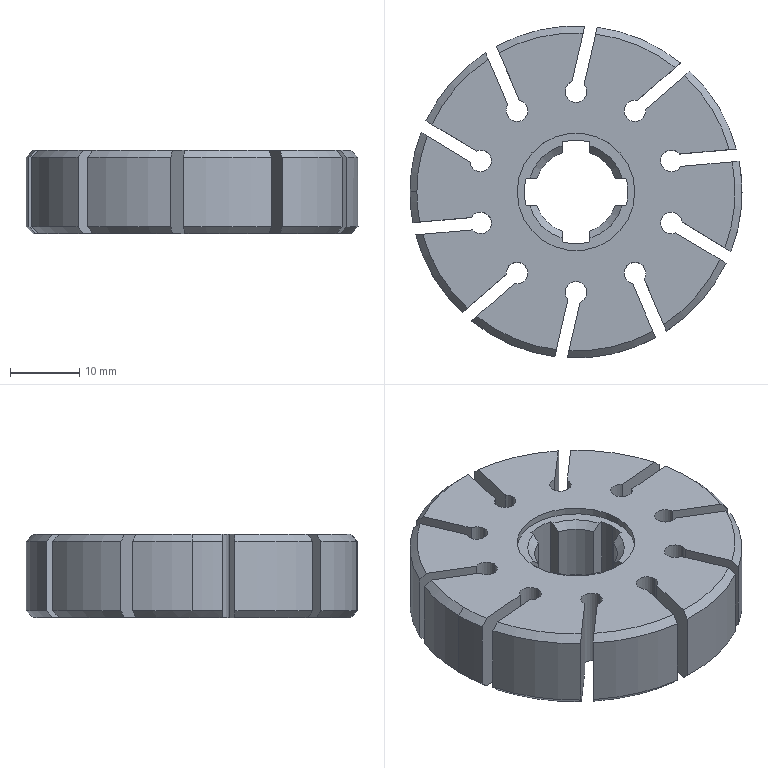Part | SolidWorks | features ICE 5, Chamfer 2, CirPattern 1, Extrusion 1 | 1 solid | 110 faces | box 48 x 48 x 12 mm | volume 17049 mm3 | cylinder 48 | plane 32 | cone 30 | commonest cylinder face diameters 3.12 x24 48 x11 15 x5 12 x4 17 x4